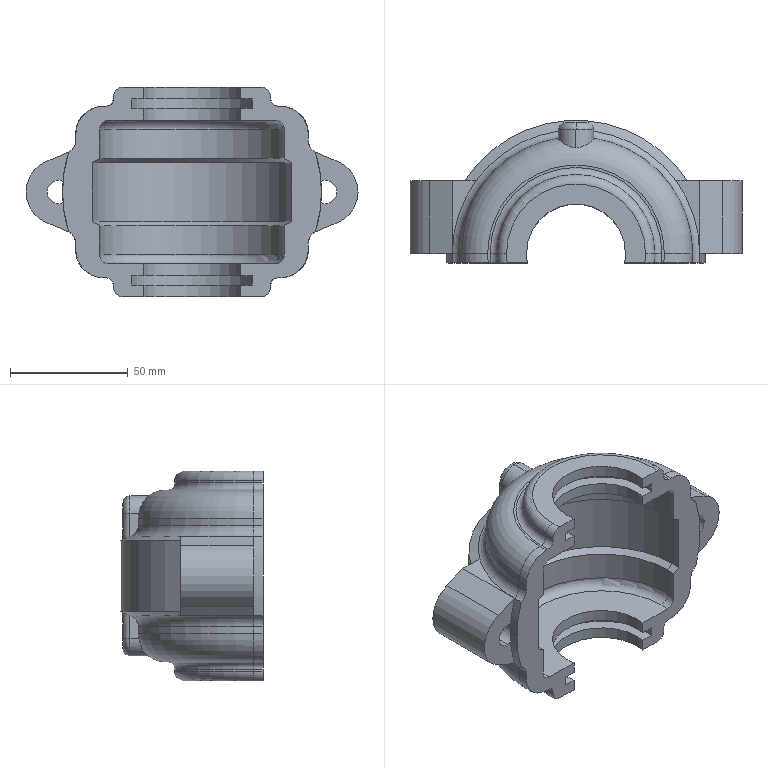Part | SolidWorks | features ICE 1, MirrorPattern 1, SplitBody 1 | 1 solid | 132 faces | box 141 x 60.5 x 89 mm | volume 190832 mm3 | cylinder 55 | plane 36 | torus 33 | cone 8 | commonest cylinder face diameters 42 x12 52 x6 67 x6 79 x6 99 x6 6 x4